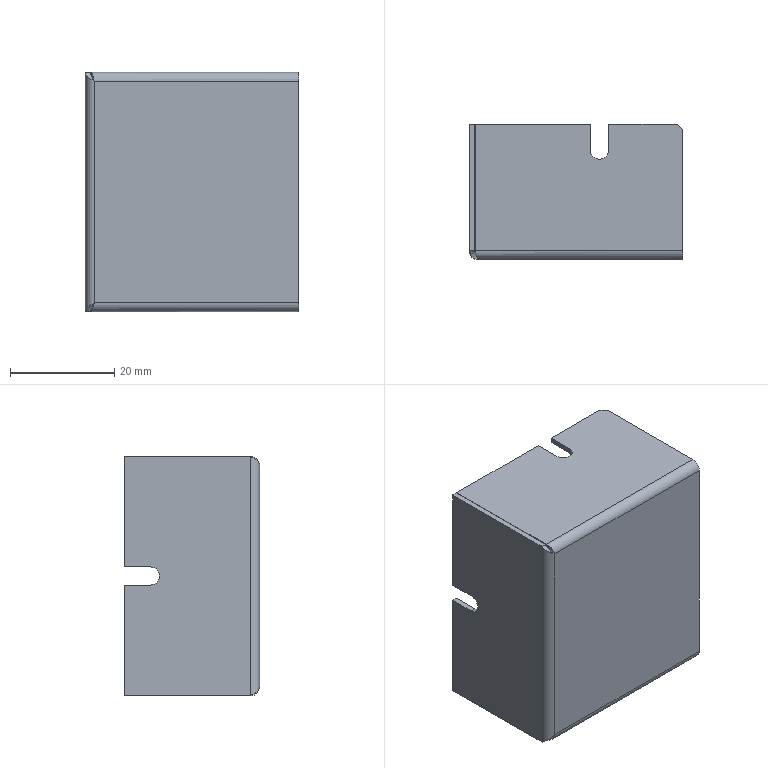Part | SolidWorks | features Chamfer 1, CornerFeat 1, Cut 1, EdgeFlange 1, FlatPattern 1, ICE 1, SMBaseFlange 1, SheetMetal 1 | 1 solid | 45 faces | box 41 x 26 x 46 mm | volume 4894 mm3 | plane 31 | cylinder 10 | spline 4 | commonest cylinder face diameters 3.5 x4 1.473 x3 3.473 x3
STEP:
#1=CARTESIAN_POINT('',(-20.,21.,23.75));
#2=VERTEX_POINT('',#1);
#3=CARTESIAN_POINT('',(-20.,19.25,22.));
#4=VERTEX_POINT('',#3);
#5=CARTESIAN_POINT('',(-20.,21.,22.));
#6=DIRECTION('',(1.,0.,0.));
#7=DIRECTION('',(0.,1.,0.));
#8=AXIS2_PLACEMENT_3D('',#5,#6,#7);
#9=CIRCLE('',#8,1.75);
#10=EDGE_CURVE('',#2,#4,#9,.T.);
#11=ORIENTED_EDGE('',*,*,#10,.T.);
#12=CARTESIAN_POINT('',(-21.,19.25,22.));
#13=VERTEX_POINT('',#12);
#14=CARTESIAN_POINT('',(-11.,19.25,22.));
#15=DIRECTION('',(-1.,0.,0.));
#16=VECTOR('',#15,1000.);
#17=LINE('',#14,#16);
#18=EDGE_CURVE('',#4,#13,#17,.T.);
#19=ORIENTED_EDGE('',*,*,#18,.T.);
#20=CARTESIAN_POINT('',(-21.,21.,23.75));
#21=VERTEX_POINT('',#20);
#22=CARTESIAN_POINT('',(-21.,21.,22.));
#23=DIRECTION('',(-1.,0.,0.));
#24=DIRECTION('',(0.,-1.,0.));
#25=AXIS2_PLACEMENT_3D('',#22,#23,#24);
#26=CIRCLE('',#25,1.75);
#27=EDGE_CURVE('',#13,#21,#26,.T.);
#28=ORIENTED_EDGE('',*,*,#27,.T.);
#29=CARTESIAN_POINT('',(-11.,21.,23.75));
#30=DIRECTION('',(-1.,0.,0.));
#31=VECTOR('',#30,1000.);
#32=LINE('',#29,#31);
#33=EDGE_CURVE('',#2,#21,#32,.T.);
#34=ORIENTED_EDGE('',*,*,#33,.F.);
#35=EDGE_LOOP('',(#11,#19,#28,#34));
#36=FACE_OUTER_BOUND('',#35,.T.);
#37=CARTESIAN_POINT('',(-11.,21.,22.));
#38=DIRECTION('',(-1.,0.,0.));
#39=DIRECTION('',(0.,-1.,0.));
#40=AXIS2_PLACEMENT_3D('',#37,#38,#39);
#41=CYLINDRICAL_SURFACE('',#40,1.75);
#42=ADVANCED_FACE('',(#36),#41,.F.);
#43=CARTESIAN_POINT('',(-20.,26.,45.));
#44=VERTEX_POINT('',#43);
#45=CARTESIAN_POINT('',(-20.,26.,23.75));
#46=VERTEX_POINT('',#45);
#47=CARTESIAN_POINT('',(-20.,26.,0.));
#48=DIRECTION('',(0.,0.,-1.));
#49=VECTOR('',#48,1000.);
#50=LINE('',#47,#49);
#51=EDGE_CURVE('',#44,#46,#50,.T.);
#52=ORIENTED_EDGE('',*,*,#51,.T.);
#53=CARTESIAN_POINT('',(-21.,26.,23.75));
#54=VERTEX_POINT('',#53);
#55=CARTESIAN_POINT('',(-21.,26.,23.75));
#56=DIRECTION('',(-1.,0.,0.));
#57=VECTOR('',#56,1000.);
#58=LINE('',#55,#57);
#59=EDGE_CURVE('',#46,#54,#58,.T.);
#60=ORIENTED_EDGE('',*,*,#59,.T.);
#61=CARTESIAN_POINT('',(-21.,26.,45.));
#62=VERTEX_POINT('',#61);
#63=CARTESIAN_POINT('',(-21.,26.,0.));
#64=DIRECTION('',(0.,0.,-1.));
#65=VECTOR('',#64,1000.);
#66=LINE('',#63,#65);
#67=EDGE_CURVE('',#62,#54,#66,.T.);
#68=ORIENTED_EDGE('',*,*,#67,.F.);
#69=CARTESIAN_POINT('',(-21.,26.,45.));
#70=DIRECTION('',(1.,0.,0.));
#71=VECTOR('',#70,1000.);
#72=LINE('',#69,#71);
#73=EDGE_CURVE('',#62,#44,#72,.T.);
#74=ORIENTED_EDGE('',*,*,#73,.T.);
#75=EDGE_LOOP('',(#52,#60,#68,#74));
#76=FACE_OUTER_BOUND('',#75,.T.);
#77=CARTESIAN_POINT('',(-21.,26.,0.));
#78=DIRECTION('',(0.,-1.,0.));
#79=DIRECTION('',(1.,0.,0.));
#80=AXIS2_PLACEMENT_3D('',#77,#78,#79);
#81=PLANE('',#80);
#82=ADVANCED_FACE('',(#76),#81,.F.);
#83=CARTESIAN_POINT('',(-19.9,26.,0.));
#84=VERTEX_POINT('',#83);
#85=CARTESIAN_POINT('',(2.25,26.,0.));
#86=VERTEX_POINT('',#85);
#87=CARTESIAN_POINT('',(20.,26.,0.));
#88=DIRECTION('',(1.,0.,0.));
#89=VECTOR('',#88,1000.);
#90=LINE('',#87,#89);
#91=EDGE_CURVE('',#84,#86,#90,.T.);
#92=ORIENTED_EDGE('',*,*,#91,.T.);
#93=CARTESIAN_POINT('',(2.25,26.,-1.));
#94=VERTEX_POINT('',#93);
#95=CARTESIAN_POINT('',(2.25,26.,-1.));
#96=DIRECTION('',(0.,0.,-1.));
#97=VECTOR('',#96,1000.);
#98=LINE('',#95,#97);
#99=EDGE_CURVE('',#86,#94,#98,.T.);
#100=ORIENTED_EDGE('',*,*,#99,.T.);
#101=CARTESIAN_POINT('',(-19.9,26.,-1.));
#102=VERTEX_POINT('',#101);
#103=CARTESIAN_POINT('',(20.,26.,-1.));
#104=DIRECTION('',(1.,0.,0.));
#105=VECTOR('',#104,1000.);
#106=LINE('',#103,#105);
#107=EDGE_CURVE('',#102,#94,#106,.T.);
#108=ORIENTED_EDGE('',*,*,#107,.F.);
#109=CARTESIAN_POINT('',(-19.9,26.,0.));
#110=DIRECTION('',(0.,0.,-1.));
#111=VECTOR('',#110,1000.);
#112=LINE('',#109,#111);
#113=EDGE_CURVE('',#84,#102,#112,.T.);
#114=ORIENTED_EDGE('',*,*,#113,.F.);
#115=EDGE_LOOP('',(#92,#100,#108,#114));
#116=FACE_OUTER_BOUND('',#115,.T.);
#117=CARTESIAN_POINT('',(20.,26.,-1.));
#118=DIRECTION('',(0.,-1.,0.));
#119=DIRECTION('',(0.,0.,-1.));
#120=AXIS2_PLACEMENT_3D('',#117,#118,#119);
#121=PLANE('',#120);
#122=ADVANCED_FACE('',(#116),#121,.F.);
#123=CARTESIAN_POINT('',(2.25,26.,45.));
#124=VERTEX_POINT('',#123);
#125=CARTESIAN_POINT('',(-19.9,26.,45.));
#126=VERTEX_POINT('',#125);
#127=CARTESIAN_POINT('',(-20.,26.,45.));
#128=DIRECTION('',(-1.,0.,0.));
#129=VECTOR('',#128,1000.);
#130=LINE('',#127,#129);
#131=EDGE_CURVE('',#124,#126,#130,.T.);
#132=ORIENTED_EDGE('',*,*,#131,.F.);
#133=CARTESIAN_POINT('',(2.25,26.,44.));
#134=VERTEX_POINT('',#133);
#135=CARTESIAN_POINT('',(2.25,26.,45.));
#136=DIRECTION('',(0.,0.,-1.));
#137=VECTOR('',#136,1000.);
#138=LINE('',#135,#137);
#139=EDGE_CURVE('',#124,#134,#138,.T.);
#140=ORIENTED_EDGE('',*,*,#139,.T.);
#141=CARTESIAN_POINT('',(-19.9,26.,44.));
#142=VERTEX_POINT('',#141);
#143=CARTESIAN_POINT('',(-20.,26.,44.));
#144=DIRECTION('',(-1.,0.,0.));
#145=VECTOR('',#144,1000.);
#146=LINE('',#143,#145);
#147=EDGE_CURVE('',#134,#142,#146,.T.);
#148=ORIENTED_EDGE('',*,*,#147,.T.);
#149=CARTESIAN_POINT('',(-19.9,26.,44.));
#150=DIRECTION('',(0.,0.,1.));
#151=VECTOR('',#150,1000.);
#152=LINE('',#149,#151);
#153=EDGE_CURVE('',#142,#126,#152,.T.);
#154=ORIENTED_EDGE('',*,*,#153,.T.);
#155=EDGE_LOOP('',(#132,#140,#148,#154));
#156=FACE_OUTER_BOUND('',#155,.T.);
#157=CARTESIAN_POINT('',(-20.,26.,45.));
#158=DIRECTION('',(0.,-1.,0.));
#159=DIRECTION('',(0.,0.,-1.));
#160=AXIS2_PLACEMENT_3D('',#157,#158,#159);
#161=PLANE('',#160);
#162=ADVANCED_FACE('',(#156),#161,.F.);
#163=CARTESIAN_POINT('',(-19.263,1.,43.263));
#164=VERTEX_POINT('',#163);
#165=CARTESIAN_POINT('',(-19.263,1.,0.7366));
#166=VERTEX_POINT('',#165);
#167=CARTESIAN_POINT('',(-19.263,1.,43.293));
#168=DIRECTION('',(0.,0.,-1.));
#169=VECTOR('',#168,1000.);
#170=LINE('',#167,#169);
#171=EDGE_CURVE('',#164,#166,#170,.T.);
#172=ORIENTED_EDGE('',*,*,#171,.F.);
#173=CARTESIAN_POINT('',(20.,1.,43.263));
#174=VERTEX_POINT('',#173);
#175=CARTESIAN_POINT('',(20.,1.,43.263));
#176=DIRECTION('',(-1.,0.,0.));
#177=VECTOR('',#176,1000.);
#178=LINE('',#175,#177);
#179=EDGE_CURVE('',#174,#164,#178,.T.);
#180=ORIENTED_EDGE('',*,*,#179,.F.);
#181=CARTESIAN_POINT('',(20.,1.,0.7366));
#182=VERTEX_POINT('',#181);
#183=CARTESIAN_POINT('',(20.,1.,44.));
#184=DIRECTION('',(0.,0.,-1.));
#185=VECTOR('',#184,1000.);
#186=LINE('',#183,#185);
#187=EDGE_CURVE('',#174,#182,#186,.T.);
#188=ORIENTED_EDGE('',*,*,#187,.T.);
#189=CARTESIAN_POINT('',(-19.293,1.,0.7366));
#190=DIRECTION('',(1.,0.,0.));
#191=VECTOR('',#190,1000.);
#192=LINE('',#189,#191);
#193=EDGE_CURVE('',#166,#182,#192,.T.);
#194=ORIENTED_EDGE('',*,*,#193,.F.);
#195=EDGE_LOOP('',(#172,#180,#188,#194));
#196=FACE_OUTER_BOUND('',#195,.T.);
#197=CARTESIAN_POINT('',(20.,1.,44.));
#198=DIRECTION('',(0.,-1.,0.));
#199=DIRECTION('',(0.,0.,-1.));
#200=AXIS2_PLACEMENT_3D('',#197,#198,#199);
#201=PLANE('',#200);
#202=ADVANCED_FACE('',(#196),#201,.F.);
#203=CARTESIAN_POINT('',(20.,0.,43.263));
#204=VERTEX_POINT('',#203);
#205=CARTESIAN_POINT('',(-19.263,0.,43.263));
#206=VERTEX_POINT('',#205);
#207=CARTESIAN_POINT('',(20.,0.,43.263));
#208=DIRECTION('',(-1.,0.,0.));
#209=VECTOR('',#208,1000.);
#210=LINE('',#207,#209);
#211=EDGE_CURVE('',#204,#206,#210,.T.);
#212=ORIENTED_EDGE('',*,*,#211,.T.);
#213=CARTESIAN_POINT('',(-19.263,0.,0.7366));
#214=VERTEX_POINT('',#213);
#215=CARTESIAN_POINT('',(-19.263,0.,43.293));
#216=DIRECTION('',(0.,0.,-1.));
#217=VECTOR('',#216,1000.);
#218=LINE('',#215,#217);
#219=EDGE_CURVE('',#206,#214,#218,.T.);
#220=ORIENTED_EDGE('',*,*,#219,.T.);
#221=CARTESIAN_POINT('',(20.,0.,0.7366));
#222=VERTEX_POINT('',#221);
#223=CARTESIAN_POINT('',(-19.293,0.,0.7366));
#224=DIRECTION('',(1.,0.,0.));
#225=VECTOR('',#224,1000.);
#226=LINE('',#223,#225);
#227=EDGE_CURVE('',#214,#222,#226,.T.);
#228=ORIENTED_EDGE('',*,*,#227,.T.);
#229=CARTESIAN_POINT('',(20.,0.,44.));
#230=DIRECTION('',(0.,0.,-1.));
#231=VECTOR('',#230,1000.);
#232=LINE('',#229,#231);
#233=EDGE_CURVE('',#204,#222,#232,.T.);
#234=ORIENTED_EDGE('',*,*,#233,.F.);
#235=EDGE_LOOP('',(#212,#220,#228,#234));
#236=FACE_OUTER_BOUND('',#235,.T.);
#237=CARTESIAN_POINT('',(20.,0.,44.));
#238=DIRECTION('',(0.,-1.,0.));
#239=DIRECTION('',(0.,0.,-1.));
#240=AXIS2_PLACEMENT_3D('',#237,#238,#239);
#241=PLANE('',#240);
#242=ADVANCED_FACE('',(#236),#241,.T.);
#243=ORIENTED_EDGE('',*,*,#187,.F.);
#244=CARTESIAN_POINT('',(20.,1.,43.263));
#245=DIRECTION('',(0.,-1.,0.));
#246=VECTOR('',#245,1000.);
#247=LINE('',#244,#246);
#248=EDGE_CURVE('',#174,#204,#247,.T.);
#249=ORIENTED_EDGE('',*,*,#248,.T.);
#250=ORIENTED_EDGE('',*,*,#233,.T.);
#251=CARTESIAN_POINT('',(20.,1.,0.7366));
#252=DIRECTION('',(0.,-1.,0.));
#253=VECTOR('',#252,1000.);
#254=LINE('',#251,#253);
#255=EDGE_CURVE('',#182,#222,#254,.T.);
#256=ORIENTED_EDGE('',*,*,#255,.F.);
#257=EDGE_LOOP('',(#243,#249,#250,#256));
#258=FACE_OUTER_BOUND('',#257,.T.);
#259=CARTESIAN_POINT('',(20.,1.,44.));
#260=DIRECTION('',(1.,0.,0.));
#261=DIRECTION('',(0.,0.,-1.));
#262=AXIS2_PLACEMENT_3D('',#259,#260,#261);
#263=PLANE('',#262);
#264=ADVANCED_FACE('',(#258),#263,.T.);
#265=CARTESIAN_POINT('',(20.,1.737,0.));
#266=VERTEX_POINT('',#265);
#267=CARTESIAN_POINT('',(20.,1.737,-1.));
#268=VERTEX_POINT('',#267);
#269=CARTESIAN_POINT('',(20.,1.737,0.));
#270=DIRECTION('',(0.,0.,-1.));
#271=VECTOR('',#270,1000.);
#272=LINE('',#269,#271);
#273=EDGE_CURVE('',#266,#268,#272,.T.);
#274=ORIENTED_EDGE('',*,*,#273,.F.);
#275=CARTESIAN_POINT('',(20.,1.737,0.7366));
#276=DIRECTION('',(-1.,0.,0.));
#277=DIRECTION('',(0.,0.,-1.));
#278=AXIS2_PLACEMENT_3D('',#275,#276,#277);
#279=CIRCLE('',#278,0.7366);
#280=EDGE_CURVE('',#266,#182,#279,.T.);
#281=ORIENTED_EDGE('',*,*,#280,.T.);
#282=ORIENTED_EDGE('',*,*,#255,.T.);
#283=CARTESIAN_POINT('',(20.,1.737,0.7366));
#284=DIRECTION('',(-1.,0.,0.));
#285=DIRECTION('',(0.,0.,1.));
#286=AXIS2_PLACEMENT_3D('',#283,#284,#285);
#287=CIRCLE('',#286,1.737);
#288=EDGE_CURVE('',#268,#222,#287,.T.);
#289=ORIENTED_EDGE('',*,*,#288,.F.);
#290=EDGE_LOOP('',(#274,#281,#282,#289));
#291=FACE_OUTER_BOUND('',#290,.T.);
#292=CARTESIAN_POINT('',(20.,1.737,0.7366));
#293=DIRECTION('',(1.,0.,0.));
#294=DIRECTION('',(0.,0.,-1.));
#295=AXIS2_PLACEMENT_3D('',#292,#293,#294);
#296=PLANE('',#295);
#297=ADVANCED_FACE('',(#291),#296,.T.);
#298=CARTESIAN_POINT('',(-19.9,1.737,0.));
#299=VERTEX_POINT('',#298);
#300=CARTESIAN_POINT('',(-19.263,1.,0.7366));
#301=CARTESIAN_POINT('',(-19.369,1.,0.5438));
#302=CARTESIAN_POINT('',(-19.476,1.079,0.3521));
#303=CARTESIAN_POINT('',(-19.688,1.352,0.07939));
#304=CARTESIAN_POINT('',(-19.794,1.544,0.));
#305=CARTESIAN_POINT('',(-19.9,1.737,0.));
#306=B_SPLINE_CURVE_WITH_KNOTS('',3,(#300,#301,#302,#303,#304,#305),.UNSPECIFIED.,.F.,.F.,(4,2,4),(0.,0.5,1.),.UNSPECIFIED.);
#307=EDGE_CURVE('',#166,#299,#306,.T.);
#308=ORIENTED_EDGE('',*,*,#307,.T.);
#309=CARTESIAN_POINT('',(-19.9,1.737,-1.));
#310=VERTEX_POINT('',#309);
#311=CARTESIAN_POINT('',(-19.9,1.737,0.));
#312=CARTESIAN_POINT('',(-19.9,1.737,-1.));
#313=B_SPLINE_CURVE_WITH_KNOTS('',1,(#311,#312),.UNSPECIFIED.,.F.,.F.,(2,2),(0.,1.),.UNSPECIFIED.);
#314=EDGE_CURVE('',#299,#310,#313,.T.);
#315=ORIENTED_EDGE('',*,*,#314,.T.);
#316=CARTESIAN_POINT('',(-19.263,0.,0.7366));
#317=CARTESIAN_POINT('',(-19.29,0.,0.622));
#318=CARTESIAN_POINT('',(-19.317,0.01124,0.5089));
#319=CARTESIAN_POINT('',(-19.37,0.05561,0.2861));
#320=CARTESIAN_POINT('',(-19.396,0.0892,0.1756));
#321=CARTESIAN_POINT('',(-19.449,0.176,-0.03353));
#322=CARTESIAN_POINT('',(-19.475,0.2293,-0.1332));
#323=CARTESIAN_POINT('',(-19.529,0.3557,-0.3226));
#324=CARTESIAN_POINT('',(-19.555,0.4287,-0.4114));
#325=CARTESIAN_POINT('',(-19.634,0.6684,-0.6511));
#326=CARTESIAN_POINT('',(-19.688,0.862,-0.7806));
#327=CARTESIAN_POINT('',(-19.793,1.28,-0.9539));
#328=CARTESIAN_POINT('',(-19.847,1.507,-1.));
#329=CARTESIAN_POINT('',(-19.9,1.737,-1.));
#330=B_SPLINE_CURVE_WITH_KNOTS('',3,(#316,#317,#318,#319,#320,#321,#322,#323,#324,#325,#326,#327,#328,#329),.UNSPECIFIED.,.F.,.F.,(4,2,2,2,2,2,4),(0.,0.0003495,0.0006991,0.001049,0.001398,0.002097,0.002796),.UNSPECIFIED.);
#331=EDGE_CURVE('',#214,#310,#330,.T.);
#332=ORIENTED_EDGE('',*,*,#331,.F.);
#333=CARTESIAN_POINT('',(-19.263,1.,0.7366));
#334=CARTESIAN_POINT('',(-19.263,0.,0.7366));
#335=B_SPLINE_CURVE_WITH_KNOTS('',1,(#333,#334),.UNSPECIFIED.,.F.,.F.,(2,2),(0.,1.),.UNSPECIFIED.);
#336=EDGE_CURVE('',#166,#214,#335,.T.);
#337=ORIENTED_EDGE('',*,*,#336,.F.);
#338=EDGE_LOOP('',(#308,#315,#332,#337));
#339=FACE_OUTER_BOUND('',#338,.T.);
#340=CARTESIAN_POINT('',(-19.263,-0.0101,0.7366));
#341=CARTESIAN_POINT('',(-19.316,-0.0101,0.5079));
#342=CARTESIAN_POINT('',(-19.37,0.03536,0.2794));
#343=CARTESIAN_POINT('',(-19.476,0.2104,-0.1431));
#344=CARTESIAN_POINT('',(-19.529,0.3398,-0.3368));
#345=CARTESIAN_POINT('',(-19.635,0.6632,-0.6602));
#346=CARTESIAN_POINT('',(-19.688,0.8569,-0.7896));
#347=CARTESIAN_POINT('',(-19.794,1.279,-0.9646));
#348=CARTESIAN_POINT('',(-19.847,1.508,-1.01));
#349=CARTESIAN_POINT('',(-19.9,1.737,-1.01));
#350=CARTESIAN_POINT('',(-19.263,0.,0.7366));
#351=CARTESIAN_POINT('',(-19.316,0.,0.5092));
#352=CARTESIAN_POINT('',(-19.37,0.0452,0.282));
#353=CARTESIAN_POINT('',(-19.476,0.2192,-0.138));
#354=CARTESIAN_POINT('',(-19.529,0.3479,-0.3306));
#355=CARTESIAN_POINT('',(-19.635,0.6694,-0.6521));
#356=CARTESIAN_POINT('',(-19.688,0.862,-0.7808));
#357=CARTESIAN_POINT('',(-19.794,1.282,-0.9548));
#358=CARTESIAN_POINT('',(-19.847,1.509,-1.));
#359=CARTESIAN_POINT('',(-19.9,1.737,-1.));
#360=CARTESIAN_POINT('',(-19.263,1.,0.7366));
#361=CARTESIAN_POINT('',(-19.316,1.,0.6402));
#362=CARTESIAN_POINT('',(-19.37,1.019,0.5438));
#363=CARTESIAN_POINT('',(-19.476,1.093,0.3656));
#364=CARTESIAN_POINT('',(-19.529,1.148,0.2839));
#365=CARTESIAN_POINT('',(-19.635,1.284,0.1476));
#366=CARTESIAN_POINT('',(-19.688,1.366,0.09297));
#367=CARTESIAN_POINT('',(-19.794,1.544,0.01917));
#368=CARTESIAN_POINT('',(-19.847,1.64,0.));
#369=CARTESIAN_POINT('',(-19.9,1.737,0.));
#370=CARTESIAN_POINT('',(-19.263,1.01,0.7366));
#371=CARTESIAN_POINT('',(-19.316,1.01,0.6415));
#372=CARTESIAN_POINT('',(-19.37,1.029,0.5464));
#373=CARTESIAN_POINT('',(-19.476,1.102,0.3707));
#374=CARTESIAN_POINT('',(-19.529,1.156,0.2901));
#375=CARTESIAN_POINT('',(-19.635,1.29,0.1556));
#376=CARTESIAN_POINT('',(-19.688,1.371,0.1017));
#377=CARTESIAN_POINT('',(-19.794,1.546,0.02891));
#378=CARTESIAN_POINT('',(-19.847,1.641,0.01));
#379=CARTESIAN_POINT('',(-19.9,1.737,0.01));
#380=B_SPLINE_SURFACE_WITH_KNOTS('',1,3,((#340,#341,#342,#343,#344,#345,#346,#347,#348,#349),(#350,#351,#352,#353,#354,#355,#356,#357,#358,#359),(#360,#361,#362,#363,#364,#365,#366,#367,#368,#369),(#370,#371,#372,#373,#374,#375,#376,#377,#378,#379)),.UNSPECIFIED.,.F.,.F.,.F.,(2,1,1,2),(4,2,2,2,4),(-0.0101,0.,1.,1.01),(0.,0.25,0.5,0.75,1.),.UNSPECIFIED.);
#381=ADVANCED_FACE('',(#339),#380,.T.);
#382=ORIENTED_EDGE('',*,*,#227,.F.);
#383=ORIENTED_EDGE('',*,*,#331,.T.);
#384=CARTESIAN_POINT('',(0.,1.737,-1.));
#385=DIRECTION('',(1.,0.,0.));
#386=VECTOR('',#385,1000.);
#387=LINE('',#384,#386);
#388=EDGE_CURVE('',#310,#268,#387,.T.);
#389=ORIENTED_EDGE('',*,*,#388,.T.);
#390=ORIENTED_EDGE('',*,*,#288,.T.);
#391=EDGE_LOOP('',(#382,#383,#389,#390));
#392=FACE_OUTER_BOUND('',#391,.T.);
#393=CARTESIAN_POINT('',(-39.591,1.737,0.7366));
#394=DIRECTION('',(1.,0.,0.));
#395=DIRECTION('',(0.,0.,-1.));
#396=AXIS2_PLACEMENT_3D('',#393,#394,#395);
#397=CYLINDRICAL_SURFACE('',#396,1.737);
#398=ADVANCED_FACE('',(#392),#397,.T.);
#399=ORIENTED_EDGE('',*,*,#193,.T.);
#400=ORIENTED_EDGE('',*,*,#280,.F.);
#401=CARTESIAN_POINT('',(20.,1.737,0.));
#402=DIRECTION('',(-1.,0.,0.));
#403=VECTOR('',#402,1000.);
#404=LINE('',#401,#403);
#405=EDGE_CURVE('',#266,#299,#404,.T.);
#406=ORIENTED_EDGE('',*,*,#405,.T.);
#407=ORIENTED_EDGE('',*,*,#307,.F.);
#408=EDGE_LOOP('',(#399,#400,#406,#407));
#409=FACE_OUTER_BOUND('',#408,.T.);
#410=CARTESIAN_POINT('',(-39.591,1.737,0.7366));
#411=DIRECTION('',(1.,0.,0.));
#412=DIRECTION('',(0.,0.,-1.));
#413=AXIS2_PLACEMENT_3D('',#410,#411,#412);
#414=CYLINDRICAL_SURFACE('',#413,0.7366);
#415=ADVANCED_FACE('',(#409),#414,.F.);
#416=CARTESIAN_POINT('',(5.75,26.,0.));
#417=VERTEX_POINT('',#416);
#418=CARTESIAN_POINT('',(19.,26.,0.));
#419=VERTEX_POINT('',#418);
#420=CARTESIAN_POINT('',(20.,26.,0.));
#421=DIRECTION('',(1.,0.,0.));
#422=VECTOR('',#421,1000.);
#423=LINE('',#420,#422);
#424=EDGE_CURVE('',#417,#419,#423,.T.);
#425=ORIENTED_EDGE('',*,*,#424,.T.);
#426=CARTESIAN_POINT('',(19.,26.,-1.));
#427=VERTEX_POINT('',#426);
#428=CARTESIAN_POINT('',(19.,26.,-1.));
#429=DIRECTION('',(0.,0.,-1.));
#430=VECTOR('',#429,1000.);
#431=LINE('',#428,#430);
#432=EDGE_CURVE('',#419,#427,#431,.T.);
#433=ORIENTED_EDGE('',*,*,#432,.T.);
#434=CARTESIAN_POINT('',(5.75,26.,-1.));
#435=VERTEX_POINT('',#434);
#436=CARTESIAN_POINT('',(20.,26.,-1.));
#437=DIRECTION('',(1.,0.,0.));
#438=VECTOR('',#437,1000.);
#439=LINE('',#436,#438);
#440=EDGE_CURVE('',#435,#427,#439,.T.);
#441=ORIENTED_EDGE('',*,*,#440,.F.);
#442=CARTESIAN_POINT('',(5.75,26.,-1.));
#443=DIRECTION('',(0.,0.,1.));
#444=VECTOR('',#443,1000.);
#445=LINE('',#442,#444);
#446=EDGE_CURVE('',#435,#417,#445,.T.);
#447=ORIENTED_EDGE('',*,*,#446,.T.);
#448=EDGE_LOOP('',(#425,#433,#441,#447));
#449=FACE_OUTER_BOUND('',#448,.T.);
#450=CARTESIAN_POINT('',(20.,26.,-1.));
#451=DIRECTION('',(0.,-1.,0.));
#452=DIRECTION('',(0.,0.,-1.));
#453=AXIS2_PLACEMENT_3D('',#450,#451,#452);
#454=PLANE('',#453);
#455=ADVANCED_FACE('',(#449),#454,.F.);
#456=ORIENTED_EDGE('',*,*,#440,.T.);
#457=CARTESIAN_POINT('',(20.,25.,-1.));
#458=VERTEX_POINT('',#457);
#459=CARTESIAN_POINT('',(20.,25.,-1.));
#460=DIRECTION('',(0.7071,-0.7071,0.));
#461=VECTOR('',#460,1000.);
#462=LINE('',#459,#461);
#463=EDGE_CURVE('',#427,#458,#462,.T.);
#464=ORIENTED_EDGE('',*,*,#463,.T.);
#465=CARTESIAN_POINT('',(20.,1.,-1.));
#466=DIRECTION('',(0.,-1.,0.));
#467=VECTOR('',#466,1000.);
#468=LINE('',#465,#467);
#469=EDGE_CURVE('',#458,#268,#468,.T.);
#470=ORIENTED_EDGE('',*,*,#469,.T.);
#471=ORIENTED_EDGE('',*,*,#388,.F.);
#472=CARTESIAN_POINT('',(-19.9,1.737,-1.));
#473=DIRECTION('',(0.,1.,0.));
#474=VECTOR('',#473,1000.);
#475=LINE('',#472,#474);
#476=EDGE_CURVE('',#310,#102,#475,.T.);
#477=ORIENTED_EDGE('',*,*,#476,.T.);
#478=ORIENTED_EDGE('',*,*,#107,.T.);
#479=CARTESIAN_POINT('',(2.25,21.,-1.));
#480=VERTEX_POINT('',#479);
#481=CARTESIAN_POINT('',(2.25,0.,-1.));
#482=DIRECTION('',(0.,-1.,0.));
#483=VECTOR('',#482,1000.);
#484=LINE('',#481,#483);
#485=EDGE_CURVE('',#94,#480,#484,.T.);
#486=ORIENTED_EDGE('',*,*,#485,.T.);
#487=CARTESIAN_POINT('',(5.75,21.,-1.));
#488=VERTEX_POINT('',#487);
#489=CARTESIAN_POINT('',(4.,21.,-1.));
#490=DIRECTION('',(0.,0.,1.));
#491=DIRECTION('',(0.,-1.,0.));
#492=AXIS2_PLACEMENT_3D('',#489,#490,#491);
#493=CIRCLE('',#492,1.75);
#494=EDGE_CURVE('',#480,#488,#493,.T.);
#495=ORIENTED_EDGE('',*,*,#494,.T.);
#496=CARTESIAN_POINT('',(5.75,0.,-1.));
#497=DIRECTION('',(0.,1.,0.));
#498=VECTOR('',#497,1000.);
#499=LINE('',#496,#498);
#500=EDGE_CURVE('',#488,#435,#499,.T.);
#501=ORIENTED_EDGE('',*,*,#500,.T.);
#502=EDGE_LOOP('',(#456,#464,#470,#471,#477,#478,#486,#495,#501));
#503=FACE_OUTER_BOUND('',#502,.T.);
#504=CARTESIAN_POINT('',(0.,0.,-1.));
#505=DIRECTION('',(0.,0.,1.));
#506=DIRECTION('',(0.,-1.,0.));
#507=AXIS2_PLACEMENT_3D('',#504,#505,#506);
#508=PLANE('',#507);
#509=ADVANCED_FACE('',(#503),#508,.F.);
#510=ORIENTED_EDGE('',*,*,#476,.F.);
#511=ORIENTED_EDGE('',*,*,#314,.F.);
#512=CARTESIAN_POINT('',(-19.9,1.737,0.));
#513=DIRECTION('',(0.,1.,0.));
#514=VECTOR('',#513,1000.);
#515=LINE('',#512,#514);
#516=EDGE_CURVE('',#299,#84,#515,.T.);
#517=ORIENTED_EDGE('',*,*,#516,.T.);
#518=ORIENTED_EDGE('',*,*,#113,.T.);
#519=EDGE_LOOP('',(#510,#511,#517,#518));
#520=FACE_OUTER_BOUND('',#519,.T.);
#521=CARTESIAN_POINT('',(-19.9,1.737,0.));
#522=DIRECTION('',(-1.,0.,0.));
#523=DIRECTION('',(0.,-1.,0.));
#524=AXIS2_PLACEMENT_3D('',#521,#522,#523);
#525=PLANE('',#524);
#526=ADVANCED_FACE('',(#520),#525,.T.);
#527=CARTESIAN_POINT('',(20.,25.,0.));
#528=VERTEX_POINT('',#527);
#529=CARTESIAN_POINT('',(20.,1.,0.));
#530=DIRECTION('',(0.,-1.,0.));
#531=VECTOR('',#530,1000.);
#532=LINE('',#529,#531);
#533=EDGE_CURVE('',#528,#266,#532,.T.);
#534=ORIENTED_EDGE('',*,*,#533,.F.);
#535=CARTESIAN_POINT('',(22.5,22.5,0.));
#536=DIRECTION('',(-0.7071,0.7071,0.));
#537=VECTOR('',#536,1000.);
#538=LINE('',#535,#537);
#539=EDGE_CURVE('',#528,#419,#538,.T.);
#540=ORIENTED_EDGE('',*,*,#539,.T.);
#541=ORIENTED_EDGE('',*,*,#424,.F.);
#542=CARTESIAN_POINT('',(5.75,21.,0.));
#543=VERTEX_POINT('',#542);
#544=CARTESIAN_POINT('',(5.75,0.,0.));
#545=DIRECTION('',(0.,1.,0.));
#546=VECTOR('',#545,1000.);
#547=LINE('',#544,#546);
#548=EDGE_CURVE('',#543,#417,#547,.T.);
#549=ORIENTED_EDGE('',*,*,#548,.F.);
#550=CARTESIAN_POINT('',(2.25,21.,0.));
#551=VERTEX_POINT('',#550);
#552=CARTESIAN_POINT('',(4.,21.,0.));
#553=DIRECTION('',(0.,0.,1.));
#554=DIRECTION('',(0.,-1.,0.));
#555=AXIS2_PLACEMENT_3D('',#552,#553,#554);
#556=CIRCLE('',#555,1.75);
#557=EDGE_CURVE('',#551,#543,#556,.T.);
#558=ORIENTED_EDGE('',*,*,#557,.F.);
#559=CARTESIAN_POINT('',(2.25,0.,0.));
#560=DIRECTION('',(0.,-1.,0.));
#561=VECTOR('',#560,1000.);
#562=LINE('',#559,#561);
#563=EDGE_CURVE('',#86,#551,#562,.T.);
#564=ORIENTED_EDGE('',*,*,#563,.F.);
#565=ORIENTED_EDGE('',*,*,#91,.F.);
#566=ORIENTED_EDGE('',*,*,#516,.F.);
#567=ORIENTED_EDGE('',*,*,#405,.F.);
#568=EDGE_LOOP('',(#534,#540,#541,#549,#558,#564,#565,#566,#567));
#569=FACE_OUTER_BOUND('',#568,.T.);
#570=CARTESIAN_POINT('',(0.,0.,0.));
#571=DIRECTION('',(0.,0.,1.));
#572=DIRECTION('',(0.,-1.,0.));
#573=AXIS2_PLACEMENT_3D('',#570,#571,#572);
#574=PLANE('',#573);
#575=ADVANCED_FACE('',(#569),#574,.T.);
#576=ORIENTED_EDGE('',*,*,#469,.F.);
#577=CARTESIAN_POINT('',(20.,25.,-1.));
#578=DIRECTION('',(0.,0.,1.));
#579=VECTOR('',#578,1000.);
#580=LINE('',#577,#579);
#581=EDGE_CURVE('',#458,#528,#580,.T.);
#582=ORIENTED_EDGE('',*,*,#581,.T.);
#583=ORIENTED_EDGE('',*,*,#533,.T.);
#584=ORIENTED_EDGE('',*,*,#273,.T.);
#585=EDGE_LOOP('',(#576,#582,#583,#584));
#586=FACE_OUTER_BOUND('',#585,.T.);
#587=CARTESIAN_POINT('',(20.,1.,-1.));
#588=DIRECTION('',(-1.,0.,0.));
#589=DIRECTION('',(0.,0.,1.));
#590=AXIS2_PLACEMENT_3D('',#587,#588,#589);
#591=PLANE('',#590);
#592=ADVANCED_FACE('',(#586),#591,.F.);
#593=CARTESIAN_POINT('',(-19.9,1.737,44.));
#594=VERTEX_POINT('',#593);
#595=CARTESIAN_POINT('',(-19.9,1.737,45.));
#596=VERTEX_POINT('',#595);
#597=CARTESIAN_POINT('',(-19.9,1.737,44.));
#598=CARTESIAN_POINT('',(-19.9,1.737,44.333));
#599=CARTESIAN_POINT('',(-19.9,1.737,44.667));
#600=CARTESIAN_POINT('',(-19.9,1.737,45.));
#601=B_SPLINE_CURVE_WITH_KNOTS('',3,(#597,#598,#599,#600),.UNSPECIFIED.,.F.,.F.,(4,4),(0.,1.),.UNSPECIFIED.);
#602=EDGE_CURVE('',#594,#596,#601,.T.);
#603=ORIENTED_EDGE('',*,*,#602,.F.);
#604=CARTESIAN_POINT('',(-19.9,1.737,44.));
#605=CARTESIAN_POINT('',(-19.794,1.544,44.));
#606=CARTESIAN_POINT('',(-19.688,1.352,43.921));
#607=CARTESIAN_POINT('',(-19.476,1.079,43.648));
#608=CARTESIAN_POINT('',(-19.37,1.,43.456));
#609=CARTESIAN_POINT('',(-19.263,1.,43.263));
#610=B_SPLINE_CURVE_WITH_KNOTS('',3,(#604,#605,#606,#607,#608,#609),.UNSPECIFIED.,.F.,.F.,(4,2,4),(0.,0.5,1.),.UNSPECIFIED.);
#611=EDGE_CURVE('',#594,#164,#610,.T.);
#612=ORIENTED_EDGE('',*,*,#611,.T.);
#613=CARTESIAN_POINT('',(-19.263,1.,43.263));
#614=CARTESIAN_POINT('',(-19.263,0.,43.263));
#615=B_SPLINE_CURVE_WITH_KNOTS('',1,(#613,#614),.UNSPECIFIED.,.F.,.F.,(2,2),(0.,1.),.UNSPECIFIED.);
#616=EDGE_CURVE('',#164,#206,#615,.T.);
#617=ORIENTED_EDGE('',*,*,#616,.T.);
#618=CARTESIAN_POINT('',(-19.9,1.737,45.));
#619=CARTESIAN_POINT('',(-19.873,1.622,45.));
#620=CARTESIAN_POINT('',(-19.847,1.509,44.989));
#621=CARTESIAN_POINT('',(-19.794,1.286,44.944));
#622=CARTESIAN_POINT('',(-19.767,1.176,44.911));
#623=CARTESIAN_POINT('',(-19.688,0.8619,44.781));
#624=CARTESIAN_POINT('',(-19.634,0.6685,44.651));
#625=CARTESIAN_POINT('',(-19.529,0.3489,44.332));
#626=CARTESIAN_POINT('',(-19.476,0.2194,44.138));
#627=CARTESIAN_POINT('',(-19.37,0.04605,43.72));
#628=CARTESIAN_POINT('',(-19.317,0.,43.493));
#629=CARTESIAN_POINT('',(-19.263,0.,43.263));
#630=B_SPLINE_CURVE_WITH_KNOTS('',3,(#618,#619,#620,#621,#622,#623,#624,#625,#626,#627,#628,#629),.UNSPECIFIED.,.F.,.F.,(4,2,2,2,2,4),(0.,0.0003496,0.0006992,0.001398,0.002098,0.002797),.UNSPECIFIED.);
#631=EDGE_CURVE('',#596,#206,#630,.T.);
#632=ORIENTED_EDGE('',*,*,#631,.F.);
#633=EDGE_LOOP('',(#603,#612,#617,#632));
#634=FACE_OUTER_BOUND('',#633,.T.);
#635=CARTESIAN_POINT('',(-19.9,1.737,45.01));
#636=CARTESIAN_POINT('',(-19.847,1.508,45.01));
#637=CARTESIAN_POINT('',(-19.794,1.279,44.965));
#638=CARTESIAN_POINT('',(-19.688,0.857,44.79));
#639=CARTESIAN_POINT('',(-19.635,0.6632,44.66));
#640=CARTESIAN_POINT('',(-19.529,0.3399,44.337));
#641=CARTESIAN_POINT('',(-19.476,0.2104,44.143));
#642=CARTESIAN_POINT('',(-19.37,0.03546,43.721));
#643=CARTESIAN_POINT('',(-19.316,-0.01,43.492));
#644=CARTESIAN_POINT('',(-19.263,-0.01,43.263));
#645=CARTESIAN_POINT('',(-19.9,1.737,45.));
#646=CARTESIAN_POINT('',(-19.847,1.509,45.));
#647=CARTESIAN_POINT('',(-19.794,1.282,44.955));
#648=CARTESIAN_POINT('',(-19.688,0.862,44.781));
#649=CARTESIAN_POINT('',(-19.635,0.6694,44.652));
#650=CARTESIAN_POINT('',(-19.529,0.3479,44.331));
#651=CARTESIAN_POINT('',(-19.476,0.2192,44.138));
#652=CARTESIAN_POINT('',(-19.37,0.0452,43.718));
#653=CARTESIAN_POINT('',(-19.316,0.,43.491));
#654=CARTESIAN_POINT('',(-19.263,0.,43.263));
#655=CARTESIAN_POINT('',(-19.9,1.737,44.));
#656=CARTESIAN_POINT('',(-19.847,1.64,44.));
#657=CARTESIAN_POINT('',(-19.794,1.544,43.981));
#658=CARTESIAN_POINT('',(-19.688,1.366,43.907));
#659=CARTESIAN_POINT('',(-19.635,1.284,43.852));
#660=CARTESIAN_POINT('',(-19.529,1.148,43.716));
#661=CARTESIAN_POINT('',(-19.476,1.093,43.634));
#662=CARTESIAN_POINT('',(-19.37,1.019,43.456));
#663=CARTESIAN_POINT('',(-19.316,1.,43.36));
#664=CARTESIAN_POINT('',(-19.263,1.,43.263));
#665=CARTESIAN_POINT('',(-19.9,1.737,43.99));
#666=CARTESIAN_POINT('',(-19.847,1.641,43.99));
#667=CARTESIAN_POINT('',(-19.794,1.546,43.971));
#668=CARTESIAN_POINT('',(-19.688,1.371,43.898));
#669=CARTESIAN_POINT('',(-19.635,1.29,43.844));
#670=CARTESIAN_POINT('',(-19.529,1.156,43.71));
#671=CARTESIAN_POINT('',(-19.476,1.102,43.629));
#672=CARTESIAN_POINT('',(-19.37,1.029,43.454));
#673=CARTESIAN_POINT('',(-19.316,1.01,43.359));
#674=CARTESIAN_POINT('',(-19.263,1.01,43.263));
#675=B_SPLINE_SURFACE_WITH_KNOTS('',1,3,((#635,#636,#637,#638,#639,#640,#641,#642,#643,#644),(#645,#646,#647,#648,#649,#650,#651,#652,#653,#654),(#655,#656,#657,#658,#659,#660,#661,#662,#663,#664),(#665,#666,#667,#668,#669,#670,#671,#672,#673,#674)),.UNSPECIFIED.,.F.,.F.,.F.,(2,1,1,2),(4,2,2,2,4),(-0.01,0.,1.,1.01),(0.,0.25,0.5,0.75,1.),.UNSPECIFIED.);
#676=ADVANCED_FACE('',(#634),#675,.T.);
#677=CARTESIAN_POINT('',(20.,1.737,44.));
#678=VERTEX_POINT('',#677);
#679=CARTESIAN_POINT('',(20.,1.737,43.263));
#680=DIRECTION('',(-1.,0.,0.));
#681=DIRECTION('',(0.,0.,1.));
#682=AXIS2_PLACEMENT_3D('',#679,#680,#681);
#683=CIRCLE('',#682,0.7366);
#684=EDGE_CURVE('',#174,#678,#683,.T.);
#685=ORIENTED_EDGE('',*,*,#684,.T.);
#686=CARTESIAN_POINT('',(20.,1.737,45.));
#687=VERTEX_POINT('',#686);
#688=CARTESIAN_POINT('',(20.,1.737,44.));
#689=DIRECTION('',(0.,0.,1.));
#690=VECTOR('',#689,1000.);
#691=LINE('',#688,#690);
#692=EDGE_CURVE('',#678,#687,#691,.T.);
#693=ORIENTED_EDGE('',*,*,#692,.T.);
#694=CARTESIAN_POINT('',(20.,1.737,43.263));
#695=DIRECTION('',(-1.,0.,0.));
#696=DIRECTION('',(0.,0.,1.));
#697=AXIS2_PLACEMENT_3D('',#694,#695,#696);
#698=CIRCLE('',#697,1.737);
#699=EDGE_CURVE('',#204,#687,#698,.T.);
#700=ORIENTED_EDGE('',*,*,#699,.F.);
#701=ORIENTED_EDGE('',*,*,#248,.F.);
#702=EDGE_LOOP('',(#685,#693,#700,#701));
#703=FACE_OUTER_BOUND('',#702,.T.);
#704=CARTESIAN_POINT('',(20.,1.737,43.263));
#705=DIRECTION('',(1.,0.,0.));
#706=DIRECTION('',(0.,0.,-1.));
#707=AXIS2_PLACEMENT_3D('',#704,#705,#706);
#708=PLANE('',#707);
#709=ADVANCED_FACE('',(#703),#708,.T.);
#710=ORIENTED_EDGE('',*,*,#211,.F.);
#711=ORIENTED_EDGE('',*,*,#699,.T.);
#712=CARTESIAN_POINT('',(0.,1.737,45.));
#713=DIRECTION('',(-1.,0.,0.));
#714=VECTOR('',#713,1000.);
#715=LINE('',#712,#714);
#716=EDGE_CURVE('',#687,#596,#715,.T.);
#717=ORIENTED_EDGE('',*,*,#716,.T.);
#718=ORIENTED_EDGE('',*,*,#631,.T.);
#719=EDGE_LOOP('',(#710,#711,#717,#718));
#720=FACE_OUTER_BOUND('',#719,.T.);
#721=CARTESIAN_POINT('',(40.328,1.737,43.263));
#722=DIRECTION('',(-1.,0.,0.));
#723=DIRECTION('',(0.,0.,1.));
#724=AXIS2_PLACEMENT_3D('',#721,#722,#723);
#725=CYLINDRICAL_SURFACE('',#724,1.737);
#726=ADVANCED_FACE('',(#720),#725,.T.);
#727=ORIENTED_EDGE('',*,*,#179,.T.);
#728=ORIENTED_EDGE('',*,*,#611,.F.);
#729=CARTESIAN_POINT('',(-20.,1.737,44.));
#730=DIRECTION('',(1.,0.,0.));
#731=VECTOR('',#730,1000.);
#732=LINE('',#729,#731);
#733=EDGE_CURVE('',#594,#678,#732,.T.);
#734=ORIENTED_EDGE('',*,*,#733,.T.);
#735=ORIENTED_EDGE('',*,*,#684,.F.);
#736=EDGE_LOOP('',(#727,#728,#734,#735));
#737=FACE_OUTER_BOUND('',#736,.T.);
#738=CARTESIAN_POINT('',(40.328,1.737,43.263));
#739=DIRECTION('',(-1.,0.,0.));
#740=DIRECTION('',(0.,0.,1.));
#741=AXIS2_PLACEMENT_3D('',#738,#739,#740);
#742=CYLINDRICAL_SURFACE('',#741,0.7366);
#743=ADVANCED_FACE('',(#737),#742,.F.);
#744=CARTESIAN_POINT('',(19.,26.,45.));
#745=VERTEX_POINT('',#744);
#746=CARTESIAN_POINT('',(5.75,26.,45.));
#747=VERTEX_POINT('',#746);
#748=CARTESIAN_POINT('',(-20.,26.,45.));
#749=DIRECTION('',(-1.,0.,0.));
#750=VECTOR('',#749,1000.);
#751=LINE('',#748,#750);
#752=EDGE_CURVE('',#745,#747,#751,.T.);
#753=ORIENTED_EDGE('',*,*,#752,.F.);
#754=CARTESIAN_POINT('',(19.,26.,44.));
#755=VERTEX_POINT('',#754);
#756=CARTESIAN_POINT('',(19.,26.,45.));
#757=DIRECTION('',(0.,0.,-1.));
#758=VECTOR('',#757,1000.);
#759=LINE('',#756,#758);
#760=EDGE_CURVE('',#745,#755,#759,.T.);
#761=ORIENTED_EDGE('',*,*,#760,.T.);
#762=CARTESIAN_POINT('',(5.75,26.,44.));
#763=VERTEX_POINT('',#762);
#764=CARTESIAN_POINT('',(-20.,26.,44.));
#765=DIRECTION('',(-1.,0.,0.));
#766=VECTOR('',#765,1000.);
#767=LINE('',#764,#766);
#768=EDGE_CURVE('',#755,#763,#767,.T.);
#769=ORIENTED_EDGE('',*,*,#768,.T.);
#770=CARTESIAN_POINT('',(5.75,26.,45.));
#771=DIRECTION('',(0.,0.,1.));
#772=VECTOR('',#771,1000.);
#773=LINE('',#770,#772);
#774=EDGE_CURVE('',#763,#747,#773,.T.);
#775=ORIENTED_EDGE('',*,*,#774,.T.);
#776=EDGE_LOOP('',(#753,#761,#769,#775));
#777=FACE_OUTER_BOUND('',#776,.T.);
#778=CARTESIAN_POINT('',(-20.,26.,45.));
#779=DIRECTION('',(0.,-1.,0.));
#780=DIRECTION('',(0.,0.,-1.));
#781=AXIS2_PLACEMENT_3D('',#778,#779,#780);
#782=PLANE('',#781);
#783=ADVANCED_FACE('',(#777),#782,.F.);
#784=CARTESIAN_POINT('',(20.,25.,45.));
#785=VERTEX_POINT('',#784);
#786=CARTESIAN_POINT('',(20.,26.,45.));
#787=DIRECTION('',(0.,1.,0.));
#788=VECTOR('',#787,1000.);
#789=LINE('',#786,#788);
#790=EDGE_CURVE('',#687,#785,#789,.T.);
#791=ORIENTED_EDGE('',*,*,#790,.T.);
#792=CARTESIAN_POINT('',(19.,26.,45.));
#793=DIRECTION('',(-0.7071,0.7071,0.));
#794=VECTOR('',#793,1000.);
#795=LINE('',#792,#794);
#796=EDGE_CURVE('',#785,#745,#795,.T.);
#797=ORIENTED_EDGE('',*,*,#796,.T.);
#798=ORIENTED_EDGE('',*,*,#752,.T.);
#799=CARTESIAN_POINT('',(5.75,21.,45.));
#800=VERTEX_POINT('',#799);
#801=CARTESIAN_POINT('',(5.75,21.,45.));
#802=DIRECTION('',(0.,1.,0.));
#803=VECTOR('',#802,1000.);
#804=LINE('',#801,#803);
#805=EDGE_CURVE('',#800,#747,#804,.T.);
#806=ORIENTED_EDGE('',*,*,#805,.F.);
#807=CARTESIAN_POINT('',(2.25,21.,45.));
#808=VERTEX_POINT('',#807);
#809=CARTESIAN_POINT('',(4.,21.,45.));
#810=DIRECTION('',(0.,0.,1.));
#811=DIRECTION('',(1.,0.,0.));
#812=AXIS2_PLACEMENT_3D('',#809,#810,#811);
#813=CIRCLE('',#812,1.75);
#814=EDGE_CURVE('',#808,#800,#813,.T.);
#815=ORIENTED_EDGE('',*,*,#814,.F.);
#816=CARTESIAN_POINT('',(2.25,21.,45.));
#817=DIRECTION('',(0.,-1.,0.));
#818=VECTOR('',#817,1000.);
#819=LINE('',#816,#818);
#820=EDGE_CURVE('',#124,#808,#819,.T.);
#821=ORIENTED_EDGE('',*,*,#820,.F.);
#822=ORIENTED_EDGE('',*,*,#131,.T.);
#823=CARTESIAN_POINT('',(-19.9,1.737,45.));
#824=DIRECTION('',(0.,1.,0.));
#825=VECTOR('',#824,1000.);
#826=LINE('',#823,#825);
#827=EDGE_CURVE('',#596,#126,#826,.T.);
#828=ORIENTED_EDGE('',*,*,#827,.F.);
#829=ORIENTED_EDGE('',*,*,#716,.F.);
#830=EDGE_LOOP('',(#791,#797,#798,#806,#815,#821,#822,#828,#829));
#831=FACE_OUTER_BOUND('',#830,.T.);
#832=CARTESIAN_POINT('',(0.,0.,45.));
#833=DIRECTION('',(0.,0.,-1.));
#834=DIRECTION('',(-1.,0.,0.));
#835=AXIS2_PLACEMENT_3D('',#832,#833,#834);
#836=PLANE('',#835);
#837=ADVANCED_FACE('',(#831),#836,.F.);
#838=CARTESIAN_POINT('',(20.,25.,44.));
#839=VERTEX_POINT('',#838);
#840=CARTESIAN_POINT('',(20.,26.,44.));
#841=DIRECTION('',(0.,1.,0.));
#842=VECTOR('',#841,1000.);
#843=LINE('',#840,#842);
#844=EDGE_CURVE('',#678,#839,#843,.T.);
#845=ORIENTED_EDGE('',*,*,#844,.T.);
#846=CARTESIAN_POINT('',(20.,25.,45.));
#847=DIRECTION('',(0.,0.,1.));
#848=VECTOR('',#847,1000.);
#849=LINE('',#846,#848);
#850=EDGE_CURVE('',#839,#785,#849,.T.);
#851=ORIENTED_EDGE('',*,*,#850,.T.);
#852=ORIENTED_EDGE('',*,*,#790,.F.);
#853=ORIENTED_EDGE('',*,*,#692,.F.);
#854=EDGE_LOOP('',(#845,#851,#852,#853));
#855=FACE_OUTER_BOUND('',#854,.T.);
#856=CARTESIAN_POINT('',(20.,26.,45.));
#857=DIRECTION('',(-1.,0.,0.));
#858=DIRECTION('',(0.,-1.,0.));
#859=AXIS2_PLACEMENT_3D('',#856,#857,#858);
#860=PLANE('',#859);
#861=ADVANCED_FACE('',(#855),#860,.F.);
#862=ORIENTED_EDGE('',*,*,#768,.F.);
#863=CARTESIAN_POINT('',(22.5,22.5,44.));
#864=DIRECTION('',(0.7071,-0.7071,0.));
#865=VECTOR('',#864,1000.);
#866=LINE('',#863,#865);
#867=EDGE_CURVE('',#755,#839,#866,.T.);
#868=ORIENTED_EDGE('',*,*,#867,.T.);
#869=ORIENTED_EDGE('',*,*,#844,.F.);
#870=ORIENTED_EDGE('',*,*,#733,.F.);
#871=CARTESIAN_POINT('',(-19.9,1.737,44.));
#872=DIRECTION('',(0.,1.,0.));
#873=VECTOR('',#872,1000.);
#874=LINE('',#871,#873);
#875=EDGE_CURVE('',#594,#142,#874,.T.);
#876=ORIENTED_EDGE('',*,*,#875,.T.);
#877=ORIENTED_EDGE('',*,*,#147,.F.);
#878=CARTESIAN_POINT('',(2.25,21.,44.));
#879=VERTEX_POINT('',#878);
#880=CARTESIAN_POINT('',(2.25,0.,44.));
#881=DIRECTION('',(0.,1.,0.));
#882=VECTOR('',#881,1000.);
#883=LINE('',#880,#882);
#884=EDGE_CURVE('',#879,#134,#883,.T.);
#885=ORIENTED_EDGE('',*,*,#884,.F.);
#886=CARTESIAN_POINT('',(5.75,21.,44.));
#887=VERTEX_POINT('',#886);
#888=CARTESIAN_POINT('',(4.,21.,44.));
#889=DIRECTION('',(0.,0.,-1.));
#890=DIRECTION('',(-1.,0.,0.));
#891=AXIS2_PLACEMENT_3D('',#888,#889,#890);
#892=CIRCLE('',#891,1.75);
#893=EDGE_CURVE('',#887,#879,#892,.T.);
#894=ORIENTED_EDGE('',*,*,#893,.F.);
#895=CARTESIAN_POINT('',(5.75,0.,44.));
#896=DIRECTION('',(0.,-1.,0.));
#897=VECTOR('',#896,1000.);
#898=LINE('',#895,#897);
#899=EDGE_CURVE('',#763,#887,#898,.T.);
#900=ORIENTED_EDGE('',*,*,#899,.F.);
#901=EDGE_LOOP('',(#862,#868,#869,#870,#876,#877,#885,#894,#900));
#902=FACE_OUTER_BOUND('',#901,.T.);
#903=CARTESIAN_POINT('',(0.,0.,44.));
#904=DIRECTION('',(0.,0.,-1.));
#905=DIRECTION('',(-1.,0.,0.));
#906=AXIS2_PLACEMENT_3D('',#903,#904,#905);
#907=PLANE('',#906);
#908=ADVANCED_FACE('',(#902),#907,.T.);
#909=ORIENTED_EDGE('',*,*,#827,.T.);
#910=ORIENTED_EDGE('',*,*,#153,.F.);
#911=ORIENTED_EDGE('',*,*,#875,.F.);
#912=ORIENTED_EDGE('',*,*,#602,.T.);
#913=EDGE_LOOP('',(#909,#910,#911,#912));
#914=FACE_OUTER_BOUND('',#913,.T.);
#915=CARTESIAN_POINT('',(-19.9,1.737,44.));
#916=DIRECTION('',(1.,0.,0.));
#917=DIRECTION('',(0.,-1.,0.));
#918=AXIS2_PLACEMENT_3D('',#915,#916,#917);
#919=PLANE('',#918);
#920=ADVANCED_FACE('',(#914),#919,.F.);
#921=CARTESIAN_POINT('',(-20.,1.737,-1.));
#922=VERTEX_POINT('',#921);
#923=CARTESIAN_POINT('',(-21.,1.737,-1.));
#924=VERTEX_POINT('',#923);
#925=CARTESIAN_POINT('',(-20.,1.737,-1.));
#926=CARTESIAN_POINT('',(-20.333,1.737,-1.));
#927=CARTESIAN_POINT('',(-20.667,1.737,-1.));
#928=CARTESIAN_POINT('',(-21.,1.737,-1.));
#929=B_SPLINE_CURVE_WITH_KNOTS('',3,(#925,#926,#927,#928),.UNSPECIFIED.,.F.,.F.,(4,4),(0.,1.),.UNSPECIFIED.);
#930=EDGE_CURVE('',#922,#924,#929,.T.);
#931=ORIENTED_EDGE('',*,*,#930,.F.);
#932=CARTESIAN_POINT('',(-20.,1.737,-1.));
#933=CARTESIAN_POINT('',(-20.,1.64,-0.8553));
#934=CARTESIAN_POINT('',(-19.981,1.544,-0.7106));
#935=CARTESIAN_POINT('',(-19.907,1.366,-0.4211));
#936=CARTESIAN_POINT('',(-19.852,1.284,-0.2764));
#937=CARTESIAN_POINT('',(-19.716,1.148,0.01302));
#938=CARTESIAN_POINT('',(-19.634,1.093,0.1577));
#939=CARTESIAN_POINT('',(-19.456,1.019,0.4472));
#940=CARTESIAN_POINT('',(-19.36,1.,0.5919));
#941=CARTESIAN_POINT('',(-19.263,1.,0.7366));
#942=B_SPLINE_CURVE_WITH_KNOTS('',3,(#932,#933,#934,#935,#936,#937,#938,#939,#940,#941),.UNSPECIFIED.,.F.,.F.,(4,2,2,2,4),(0.,0.25,0.5,0.75,1.),.UNSPECIFIED.);
#943=EDGE_CURVE('',#922,#166,#942,.T.);
#944=ORIENTED_EDGE('',*,*,#943,.T.);
#945=ORIENTED_EDGE('',*,*,#336,.T.);
#946=CARTESIAN_POINT('',(-21.,1.737,-1.));
#947=CARTESIAN_POINT('',(-21.,1.509,-0.8553));
#948=CARTESIAN_POINT('',(-20.955,1.282,-0.7106));
#949=CARTESIAN_POINT('',(-20.781,0.862,-0.4211));
#950=CARTESIAN_POINT('',(-20.652,0.6694,-0.2764));
#951=CARTESIAN_POINT('',(-20.331,0.3479,0.01302));
#952=CARTESIAN_POINT('',(-20.138,0.2192,0.1577));
#953=CARTESIAN_POINT('',(-19.718,0.0452,0.4472));
#954=CARTESIAN_POINT('',(-19.491,0.,0.5919));
#955=CARTESIAN_POINT('',(-19.263,0.,0.7366));
#956=B_SPLINE_CURVE_WITH_KNOTS('',3,(#946,#947,#948,#949,#950,#951,#952,#953,#954,#955),.UNSPECIFIED.,.F.,.F.,(4,2,2,2,4),(0.,0.25,0.5,0.75,1.),.UNSPECIFIED.);
#957=EDGE_CURVE('',#924,#214,#956,.T.);
#958=ORIENTED_EDGE('',*,*,#957,.F.);
#959=EDGE_LOOP('',(#931,#944,#945,#958));
#960=FACE_OUTER_BOUND('',#959,.T.);
#961=CARTESIAN_POINT('',(-21.,1.737,-1.));
#962=CARTESIAN_POINT('',(-21.,1.509,-0.8553));
#963=CARTESIAN_POINT('',(-20.955,1.282,-0.7106));
#964=CARTESIAN_POINT('',(-20.781,0.862,-0.4211));
#965=CARTESIAN_POINT('',(-20.652,0.6694,-0.2764));
#966=CARTESIAN_POINT('',(-20.331,0.3479,0.01302));
#967=CARTESIAN_POINT('',(-20.138,0.2192,0.1577));
#968=CARTESIAN_POINT('',(-19.718,0.0452,0.4472));
#969=CARTESIAN_POINT('',(-19.491,0.,0.5919));
#970=CARTESIAN_POINT('',(-19.263,0.,0.7366));
#971=CARTESIAN_POINT('',(-20.,1.737,-1.));
#972=CARTESIAN_POINT('',(-20.,1.64,-0.8553));
#973=CARTESIAN_POINT('',(-19.981,1.544,-0.7106));
#974=CARTESIAN_POINT('',(-19.907,1.366,-0.4211));
#975=CARTESIAN_POINT('',(-19.852,1.284,-0.2764));
#976=CARTESIAN_POINT('',(-19.716,1.148,0.01302));
#977=CARTESIAN_POINT('',(-19.634,1.093,0.1577));
#978=CARTESIAN_POINT('',(-19.456,1.019,0.4472));
#979=CARTESIAN_POINT('',(-19.36,1.,0.5919));
#980=CARTESIAN_POINT('',(-19.263,1.,0.7366));
#981=B_SPLINE_SURFACE_WITH_KNOTS('',1,3,((#961,#962,#963,#964,#965,#966,#967,#968,#969,#970),(#971,#972,#973,#974,#975,#976,#977,#978,#979,#980)),.UNSPECIFIED.,.F.,.F.,.F.,(2,2),(4,2,2,2,4),(0.,1.),(0.,0.25,0.5,0.75,1.),.UNSPECIFIED.);
#982=ADVANCED_FACE('',(#960),#981,.T.);
#983=CARTESIAN_POINT('',(-20.,1.737,45.));
#984=VERTEX_POINT('',#983);
#985=CARTESIAN_POINT('',(-19.263,1.,43.263));
#986=CARTESIAN_POINT('',(-19.36,1.,43.408));
#987=CARTESIAN_POINT('',(-19.456,1.019,43.553));
#988=CARTESIAN_POINT('',(-19.634,1.093,43.842));
#989=CARTESIAN_POINT('',(-19.716,1.148,43.987));
#990=CARTESIAN_POINT('',(-19.852,1.284,44.276));
#991=CARTESIAN_POINT('',(-19.907,1.366,44.421));
#992=CARTESIAN_POINT('',(-19.981,1.544,44.711));
#993=CARTESIAN_POINT('',(-20.,1.64,44.855));
#994=CARTESIAN_POINT('',(-20.,1.737,45.));
#995=B_SPLINE_CURVE_WITH_KNOTS('',3,(#985,#986,#987,#988,#989,#990,#991,#992,#993,#994),.UNSPECIFIED.,.F.,.F.,(4,2,2,2,4),(0.,0.25,0.5,0.75,1.),.UNSPECIFIED.);
#996=EDGE_CURVE('',#164,#984,#995,.T.);
#997=ORIENTED_EDGE('',*,*,#996,.T.);
#998=CARTESIAN_POINT('',(-21.,1.737,45.));
#999=VERTEX_POINT('',#998);
#1000=CARTESIAN_POINT('',(-21.,1.737,45.));
#1001=CARTESIAN_POINT('',(-20.667,1.737,45.));
#1002=CARTESIAN_POINT('',(-20.333,1.737,45.));
#1003=CARTESIAN_POINT('',(-20.,1.737,45.));
#1004=B_SPLINE_CURVE_WITH_KNOTS('',3,(#1000,#1001,#1002,#1003),.UNSPECIFIED.,.F.,.F.,(4,4),(0.,1.),.UNSPECIFIED.);
#1005=EDGE_CURVE('',#999,#984,#1004,.T.);
#1006=ORIENTED_EDGE('',*,*,#1005,.F.);
#1007=CARTESIAN_POINT('',(-19.263,0.,43.263));
#1008=CARTESIAN_POINT('',(-19.491,0.,43.408));
#1009=CARTESIAN_POINT('',(-19.718,0.0452,43.553));
#1010=CARTESIAN_POINT('',(-20.138,0.2192,43.842));
#1011=CARTESIAN_POINT('',(-20.331,0.3479,43.987));
#1012=CARTESIAN_POINT('',(-20.652,0.6694,44.276));
#1013=CARTESIAN_POINT('',(-20.781,0.862,44.421));
#1014=CARTESIAN_POINT('',(-20.955,1.282,44.711));
#1015=CARTESIAN_POINT('',(-21.,1.509,44.855));
#1016=CARTESIAN_POINT('',(-21.,1.737,45.));
#1017=B_SPLINE_CURVE_WITH_KNOTS('',3,(#1007,#1008,#1009,#1010,#1011,#1012,#1013,#1014,#1015,#1016),.UNSPECIFIED.,.F.,.F.,(4,2,2,2,4),(0.,0.25,0.5,0.75,1.),.UNSPECIFIED.);
#1018=EDGE_CURVE('',#206,#999,#1017,.T.);
#1019=ORIENTED_EDGE('',*,*,#1018,.F.);
#1020=ORIENTED_EDGE('',*,*,#616,.F.);
#1021=EDGE_LOOP('',(#997,#1006,#1019,#1020));
#1022=FACE_OUTER_BOUND('',#1021,.T.);
#1023=CARTESIAN_POINT('',(-19.263,0.,43.263));
#1024=CARTESIAN_POINT('',(-19.491,0.,43.408));
#1025=CARTESIAN_POINT('',(-19.718,0.0452,43.553));
#1026=CARTESIAN_POINT('',(-20.138,0.2192,43.842));
#1027=CARTESIAN_POINT('',(-20.331,0.3479,43.987));
#1028=CARTESIAN_POINT('',(-20.652,0.6694,44.276));
#1029=CARTESIAN_POINT('',(-20.781,0.862,44.421));
#1030=CARTESIAN_POINT('',(-20.955,1.282,44.711));
#1031=CARTESIAN_POINT('',(-21.,1.509,44.855));
#1032=CARTESIAN_POINT('',(-21.,1.737,45.));
#1033=CARTESIAN_POINT('',(-19.263,1.,43.263));
#1034=CARTESIAN_POINT('',(-19.36,1.,43.408));
#1035=CARTESIAN_POINT('',(-19.456,1.019,43.553));
#1036=CARTESIAN_POINT('',(-19.634,1.093,43.842));
#1037=CARTESIAN_POINT('',(-19.716,1.148,43.987));
#1038=CARTESIAN_POINT('',(-19.852,1.284,44.276));
#1039=CARTESIAN_POINT('',(-19.907,1.366,44.421));
#1040=CARTESIAN_POINT('',(-19.981,1.544,44.711));
#1041=CARTESIAN_POINT('',(-20.,1.64,44.855));
#1042=CARTESIAN_POINT('',(-20.,1.737,45.));
#1043=B_SPLINE_SURFACE_WITH_KNOTS('',1,3,((#1023,#1024,#1025,#1026,#1027,#1028,#1029,#1030,#1031,#1032),(#1033,#1034,#1035,#1036,#1037,#1038,#1039,#1040,#1041,#1042)),.UNSPECIFIED.,.F.,.F.,.F.,(2,2),(4,2,2,2,4),(0.,1.),(0.,0.25,0.5,0.75,1.),.UNSPECIFIED.);
#1044=ADVANCED_FACE('',(#1022),#1043,.T.);
#1045=ORIENTED_EDGE('',*,*,#219,.F.);
#1046=ORIENTED_EDGE('',*,*,#1018,.T.);
#1047=CARTESIAN_POINT('',(-21.,1.737,0.));
#1048=DIRECTION('',(0.,0.,-1.));
#1049=VECTOR('',#1048,1000.);
#1050=LINE('',#1047,#1049);
#1051=EDGE_CURVE('',#999,#924,#1050,.T.);
#1052=ORIENTED_EDGE('',*,*,#1051,.T.);
#1053=ORIENTED_EDGE('',*,*,#957,.T.);
#1054=EDGE_LOOP('',(#1045,#1046,#1052,#1053));
#1055=FACE_OUTER_BOUND('',#1054,.T.);
#1056=CARTESIAN_POINT('',(-19.263,1.737,68.052));
#1057=DIRECTION('',(0.,0.,-1.));
#1058=DIRECTION('',(-1.,0.,0.));
#1059=AXIS2_PLACEMENT_3D('',#1056,#1057,#1058);
#1060=CYLINDRICAL_SURFACE('',#1059,1.737);
#1061=ADVANCED_FACE('',(#1055),#1060,.T.);
#1062=ORIENTED_EDGE('',*,*,#171,.T.);
#1063=ORIENTED_EDGE('',*,*,#943,.F.);
#1064=CARTESIAN_POINT('',(-20.,1.737,0.));
#1065=DIRECTION('',(0.,0.,1.));
#1066=VECTOR('',#1065,1000.);
#1067=LINE('',#1064,#1066);
#1068=EDGE_CURVE('',#922,#984,#1067,.T.);
#1069=ORIENTED_EDGE('',*,*,#1068,.T.);
#1070=ORIENTED_EDGE('',*,*,#996,.F.);
#1071=EDGE_LOOP('',(#1062,#1063,#1069,#1070));
#1072=FACE_OUTER_BOUND('',#1071,.T.);
#1073=CARTESIAN_POINT('',(-19.263,1.737,68.052));
#1074=DIRECTION('',(0.,0.,-1.));
#1075=DIRECTION('',(-1.,0.,0.));
#1076=AXIS2_PLACEMENT_3D('',#1073,#1074,#1075);
#1077=CYLINDRICAL_SURFACE('',#1076,0.7366);
#1078=ADVANCED_FACE('',(#1072),#1077,.F.);
#1079=CARTESIAN_POINT('',(-21.,26.,20.25));
#1080=VERTEX_POINT('',#1079);
#1081=CARTESIAN_POINT('',(-21.,26.,-1.));
#1082=VERTEX_POINT('',#1081);
#1083=CARTESIAN_POINT('',(-21.,26.,0.));
#1084=DIRECTION('',(0.,0.,-1.));
#1085=VECTOR('',#1084,1000.);
#1086=LINE('',#1083,#1085);
#1087=EDGE_CURVE('',#1080,#1082,#1086,.T.);
#1088=ORIENTED_EDGE('',*,*,#1087,.F.);
#1089=CARTESIAN_POINT('',(-20.,26.,20.25));
#1090=VERTEX_POINT('',#1089);
#1091=CARTESIAN_POINT('',(-21.,26.,20.25));
#1092=DIRECTION('',(1.,0.,0.));
#1093=VECTOR('',#1092,1000.);
#1094=LINE('',#1091,#1093);
#1095=EDGE_CURVE('',#1080,#1090,#1094,.T.);
#1096=ORIENTED_EDGE('',*,*,#1095,.T.);
#1097=CARTESIAN_POINT('',(-20.,26.,-1.));
#1098=VERTEX_POINT('',#1097);
#1099=CARTESIAN_POINT('',(-20.,26.,0.));
#1100=DIRECTION('',(0.,0.,-1.));
#1101=VECTOR('',#1100,1000.);
#1102=LINE('',#1099,#1101);
#1103=EDGE_CURVE('',#1090,#1098,#1102,.T.);
#1104=ORIENTED_EDGE('',*,*,#1103,.T.);
#1105=CARTESIAN_POINT('',(-21.,26.,-1.));
#1106=DIRECTION('',(1.,0.,0.));
#1107=VECTOR('',#1106,1000.);
#1108=LINE('',#1105,#1107);
#1109=EDGE_CURVE('',#1082,#1098,#1108,.T.);
#1110=ORIENTED_EDGE('',*,*,#1109,.F.);
#1111=EDGE_LOOP('',(#1088,#1096,#1104,#1110));
#1112=FACE_OUTER_BOUND('',#1111,.T.);
#1113=CARTESIAN_POINT('',(-21.,26.,0.));
#1114=DIRECTION('',(0.,-1.,0.));
#1115=DIRECTION('',(1.,0.,0.));
#1116=AXIS2_PLACEMENT_3D('',#1113,#1114,#1115);
#1117=PLANE('',#1116);
#1118=ADVANCED_FACE('',(#1112),#1117,.F.);
#1119=ORIENTED_EDGE('',*,*,#67,.T.);
#1120=CARTESIAN_POINT('',(-21.,31.,23.75));
#1121=DIRECTION('',(0.,1.,0.));
#1122=VECTOR('',#1121,1000.);
#1123=LINE('',#1120,#1122);
#1124=EDGE_CURVE('',#21,#54,#1123,.T.);
#1125=ORIENTED_EDGE('',*,*,#1124,.F.);
#1126=ORIENTED_EDGE('',*,*,#27,.F.);
#1127=CARTESIAN_POINT('',(-21.,21.,20.25));
#1128=VERTEX_POINT('',#1127);
#1129=CARTESIAN_POINT('',(-21.,21.,22.));
#1130=DIRECTION('',(-1.,0.,0.));
#1131=DIRECTION('',(0.,-1.,0.));
#1132=AXIS2_PLACEMENT_3D('',#1129,#1130,#1131);
#1133=CIRCLE('',#1132,1.75);
#1134=EDGE_CURVE('',#1128,#13,#1133,.T.);
#1135=ORIENTED_EDGE('',*,*,#1134,.F.);
#1136=CARTESIAN_POINT('',(-21.,31.,20.25));
#1137=DIRECTION('',(0.,-1.,0.));
#1138=VECTOR('',#1137,1000.);
#1139=LINE('',#1136,#1138);
#1140=EDGE_CURVE('',#1080,#1128,#1139,.T.);
#1141=ORIENTED_EDGE('',*,*,#1140,.F.);
#1142=ORIENTED_EDGE('',*,*,#1087,.T.);
#1143=CARTESIAN_POINT('',(-21.,1.737,-1.));
#1144=DIRECTION('',(0.,1.,0.));
#1145=VECTOR('',#1144,1000.);
#1146=LINE('',#1143,#1145);
#1147=EDGE_CURVE('',#924,#1082,#1146,.T.);
#1148=ORIENTED_EDGE('',*,*,#1147,.F.);
#1149=ORIENTED_EDGE('',*,*,#1051,.F.);
#1150=CARTESIAN_POINT('',(-21.,1.737,45.));
#1151=DIRECTION('',(0.,1.,0.));
#1152=VECTOR('',#1151,1000.);
#1153=LINE('',#1150,#1152);
#1154=EDGE_CURVE('',#999,#62,#1153,.T.);
#1155=ORIENTED_EDGE('',*,*,#1154,.T.);
#1156=EDGE_LOOP('',(#1119,#1125,#1126,#1135,#1141,#1142,#1148,#1149,#1155));
#1157=FACE_OUTER_BOUND('',#1156,.T.);
#1158=CARTESIAN_POINT('',(-21.,0.,0.));
#1159=DIRECTION('',(1.,0.,0.));
#1160=DIRECTION('',(0.,1.,0.));
#1161=AXIS2_PLACEMENT_3D('',#1158,#1159,#1160);
#1162=PLANE('',#1161);
#1163=ADVANCED_FACE('',(#1157),#1162,.F.);
#1164=CARTESIAN_POINT('',(-20.,1.737,45.));
#1165=DIRECTION('',(0.,1.,0.));
#1166=VECTOR('',#1165,1000.);
#1167=LINE('',#1164,#1166);
#1168=EDGE_CURVE('',#984,#44,#1167,.T.);
#1169=ORIENTED_EDGE('',*,*,#1168,.T.);
#1170=ORIENTED_EDGE('',*,*,#73,.F.);
#1171=ORIENTED_EDGE('',*,*,#1154,.F.);
#1172=ORIENTED_EDGE('',*,*,#1005,.T.);
#1173=EDGE_LOOP('',(#1169,#1170,#1171,#1172));
#1174=FACE_OUTER_BOUND('',#1173,.T.);
#1175=CARTESIAN_POINT('',(-21.,1.737,45.));
#1176=DIRECTION('',(0.,0.,-1.));
#1177=DIRECTION('',(0.,1.,0.));
#1178=AXIS2_PLACEMENT_3D('',#1175,#1176,#1177);
#1179=PLANE('',#1178);
#1180=ADVANCED_FACE('',(#1174),#1179,.F.);
#1181=CARTESIAN_POINT('',(-20.,0.,23.75));
#1182=DIRECTION('',(0.,-1.,0.));
#1183=VECTOR('',#1182,1000.);
#1184=LINE('',#1181,#1183);
#1185=EDGE_CURVE('',#46,#2,#1184,.T.);
#1186=ORIENTED_EDGE('',*,*,#1185,.F.);
#1187=ORIENTED_EDGE('',*,*,#51,.F.);
#1188=ORIENTED_EDGE('',*,*,#1168,.F.);
#1189=ORIENTED_EDGE('',*,*,#1068,.F.);
#1190=CARTESIAN_POINT('',(-20.,1.737,-1.));
#1191=DIRECTION('',(0.,1.,0.));
#1192=VECTOR('',#1191,1000.);
#1193=LINE('',#1190,#1192);
#1194=EDGE_CURVE('',#922,#1098,#1193,.T.);
#1195=ORIENTED_EDGE('',*,*,#1194,.T.);
#1196=ORIENTED_EDGE('',*,*,#1103,.F.);
#1197=CARTESIAN_POINT('',(-20.,21.,20.25));
#1198=VERTEX_POINT('',#1197);
#1199=CARTESIAN_POINT('',(-20.,0.,20.25));
#1200=DIRECTION('',(0.,1.,0.));
#1201=VECTOR('',#1200,1000.);
#1202=LINE('',#1199,#1201);
#1203=EDGE_CURVE('',#1198,#1090,#1202,.T.);
#1204=ORIENTED_EDGE('',*,*,#1203,.F.);
#1205=CARTESIAN_POINT('',(-20.,21.,22.));
#1206=DIRECTION('',(1.,0.,0.));
#1207=DIRECTION('',(0.,1.,0.));
#1208=AXIS2_PLACEMENT_3D('',#1205,#1206,#1207);
#1209=CIRCLE('',#1208,1.75);
#1210=EDGE_CURVE('',#4,#1198,#1209,.T.);
#1211=ORIENTED_EDGE('',*,*,#1210,.F.);
#1212=ORIENTED_EDGE('',*,*,#10,.F.);
#1213=EDGE_LOOP('',(#1186,#1187,#1188,#1189,#1195,#1196,#1204,#1211,#1212));
#1214=FACE_OUTER_BOUND('',#1213,.T.);
#1215=CARTESIAN_POINT('',(-20.,0.,0.));
#1216=DIRECTION('',(1.,0.,0.));
#1217=DIRECTION('',(0.,1.,0.));
#1218=AXIS2_PLACEMENT_3D('',#1215,#1216,#1217);
#1219=PLANE('',#1218);
#1220=ADVANCED_FACE('',(#1214),#1219,.T.);
#1221=ORIENTED_EDGE('',*,*,#1194,.F.);
#1222=ORIENTED_EDGE('',*,*,#930,.T.);
#1223=ORIENTED_EDGE('',*,*,#1147,.T.);
#1224=ORIENTED_EDGE('',*,*,#1109,.T.);
#1225=EDGE_LOOP('',(#1221,#1222,#1223,#1224));
#1226=FACE_OUTER_BOUND('',#1225,.T.);
#1227=CARTESIAN_POINT('',(-21.,1.737,-1.));
#1228=DIRECTION('',(0.,0.,-1.));
#1229=DIRECTION('',(0.,1.,0.));
#1230=AXIS2_PLACEMENT_3D('',#1227,#1228,#1229);
#1231=PLANE('',#1230);
#1232=ADVANCED_FACE('',(#1226),#1231,.T.);
#1233=ORIENTED_EDGE('',*,*,#820,.T.);
#1234=CARTESIAN_POINT('',(2.25,21.,-1.003));
#1235=DIRECTION('',(0.,0.,1.));
#1236=VECTOR('',#1235,1000.);
#1237=LINE('',#1234,#1236);
#1238=EDGE_CURVE('',#879,#808,#1237,.T.);
#1239=ORIENTED_EDGE('',*,*,#1238,.F.);
#1240=ORIENTED_EDGE('',*,*,#884,.T.);
#1241=ORIENTED_EDGE('',*,*,#139,.F.);
#1242=EDGE_LOOP('',(#1233,#1239,#1240,#1241));
#1243=FACE_OUTER_BOUND('',#1242,.T.);
#1244=CARTESIAN_POINT('',(2.25,21.,-1.003));
#1245=DIRECTION('',(-1.,0.,0.));
#1246=DIRECTION('',(0.,0.,1.));
#1247=AXIS2_PLACEMENT_3D('',#1244,#1245,#1246);
#1248=PLANE('',#1247);
#1249=ADVANCED_FACE('',(#1243),#1248,.F.);
#1250=ORIENTED_EDGE('',*,*,#899,.T.);
#1251=CARTESIAN_POINT('',(5.75,21.,-1.003));
#1252=DIRECTION('',(0.,0.,1.));
#1253=VECTOR('',#1252,1000.);
#1254=LINE('',#1251,#1253);
#1255=EDGE_CURVE('',#887,#800,#1254,.T.);
#1256=ORIENTED_EDGE('',*,*,#1255,.T.);
#1257=ORIENTED_EDGE('',*,*,#805,.T.);
#1258=ORIENTED_EDGE('',*,*,#774,.F.);
#1259=EDGE_LOOP('',(#1250,#1256,#1257,#1258));
#1260=FACE_OUTER_BOUND('',#1259,.T.);
#1261=CARTESIAN_POINT('',(5.75,21.,-1.003));
#1262=DIRECTION('',(1.,0.,0.));
#1263=DIRECTION('',(0.,0.,-1.));
#1264=AXIS2_PLACEMENT_3D('',#1261,#1262,#1263);
#1265=PLANE('',#1264);
#1266=ADVANCED_FACE('',(#1260),#1265,.F.);
#1267=ORIENTED_EDGE('',*,*,#893,.T.);
#1268=ORIENTED_EDGE('',*,*,#1238,.T.);
#1269=ORIENTED_EDGE('',*,*,#814,.T.);
#1270=ORIENTED_EDGE('',*,*,#1255,.F.);
#1271=EDGE_LOOP('',(#1267,#1268,#1269,#1270));
#1272=FACE_OUTER_BOUND('',#1271,.T.);
#1273=CARTESIAN_POINT('',(4.,21.,-1.003));
#1274=DIRECTION('',(0.,0.,1.));
#1275=DIRECTION('',(1.,0.,0.));
#1276=AXIS2_PLACEMENT_3D('',#1273,#1274,#1275);
#1277=CYLINDRICAL_SURFACE('',#1276,1.75);
#1278=ADVANCED_FACE('',(#1272),#1277,.F.);
#1279=CARTESIAN_POINT('',(2.25,21.,-1.003));
#1280=DIRECTION('',(0.,0.,1.));
#1281=VECTOR('',#1280,1000.);
#1282=LINE('',#1279,#1281);
#1283=EDGE_CURVE('',#480,#551,#1282,.T.);
#1284=ORIENTED_EDGE('',*,*,#1283,.T.);
#1285=ORIENTED_EDGE('',*,*,#557,.T.);
#1286=CARTESIAN_POINT('',(5.75,21.,-1.003));
#1287=DIRECTION('',(0.,0.,1.));
#1288=VECTOR('',#1287,1000.);
#1289=LINE('',#1286,#1288);
#1290=EDGE_CURVE('',#488,#543,#1289,.T.);
#1291=ORIENTED_EDGE('',*,*,#1290,.F.);
#1292=ORIENTED_EDGE('',*,*,#494,.F.);
#1293=EDGE_LOOP('',(#1284,#1285,#1291,#1292));
#1294=FACE_OUTER_BOUND('',#1293,.T.);
#1295=CARTESIAN_POINT('',(4.,21.,-1.003));
#1296=DIRECTION('',(0.,0.,1.));
#1297=DIRECTION('',(1.,0.,0.));
#1298=AXIS2_PLACEMENT_3D('',#1295,#1296,#1297);
#1299=CYLINDRICAL_SURFACE('',#1298,1.75);
#1300=ADVANCED_FACE('',(#1294),#1299,.F.);
#1301=ORIENTED_EDGE('',*,*,#99,.F.);
#1302=ORIENTED_EDGE('',*,*,#563,.T.);
#1303=ORIENTED_EDGE('',*,*,#1283,.F.);
#1304=ORIENTED_EDGE('',*,*,#485,.F.);
#1305=EDGE_LOOP('',(#1301,#1302,#1303,#1304));
#1306=FACE_OUTER_BOUND('',#1305,.T.);
#1307=CARTESIAN_POINT('',(2.25,21.,-1.003));
#1308=DIRECTION('',(-1.,0.,0.));
#1309=DIRECTION('',(0.,0.,1.));
#1310=AXIS2_PLACEMENT_3D('',#1307,#1308,#1309);
#1311=PLANE('',#1310);
#1312=ADVANCED_FACE('',(#1306),#1311,.F.);
#1313=ORIENTED_EDGE('',*,*,#1290,.T.);
#1314=ORIENTED_EDGE('',*,*,#548,.T.);
#1315=ORIENTED_EDGE('',*,*,#446,.F.);
#1316=ORIENTED_EDGE('',*,*,#500,.F.);
#1317=EDGE_LOOP('',(#1313,#1314,#1315,#1316));
#1318=FACE_OUTER_BOUND('',#1317,.T.);
#1319=CARTESIAN_POINT('',(5.75,21.,-1.003));
#1320=DIRECTION('',(1.,0.,0.));
#1321=DIRECTION('',(0.,0.,-1.));
#1322=AXIS2_PLACEMENT_3D('',#1319,#1320,#1321);
#1323=PLANE('',#1322);
#1324=ADVANCED_FACE('',(#1318),#1323,.F.);
#1325=ORIENTED_EDGE('',*,*,#1185,.T.);
#1326=ORIENTED_EDGE('',*,*,#33,.T.);
#1327=ORIENTED_EDGE('',*,*,#1124,.T.);
#1328=ORIENTED_EDGE('',*,*,#59,.F.);
#1329=EDGE_LOOP('',(#1325,#1326,#1327,#1328));
#1330=FACE_OUTER_BOUND('',#1329,.T.);
#1331=CARTESIAN_POINT('',(-11.,31.,23.75));
#1332=DIRECTION('',(0.,0.,1.));
#1333=DIRECTION('',(0.,-1.,0.));
#1334=AXIS2_PLACEMENT_3D('',#1331,#1332,#1333);
#1335=PLANE('',#1334);
#1336=ADVANCED_FACE('',(#1330),#1335,.F.);
#1337=ORIENTED_EDGE('',*,*,#1140,.T.);
#1338=CARTESIAN_POINT('',(-11.,21.,20.25));
#1339=DIRECTION('',(-1.,0.,0.));
#1340=VECTOR('',#1339,1000.);
#1341=LINE('',#1338,#1340);
#1342=EDGE_CURVE('',#1198,#1128,#1341,.T.);
#1343=ORIENTED_EDGE('',*,*,#1342,.F.);
#1344=ORIENTED_EDGE('',*,*,#1203,.T.);
#1345=ORIENTED_EDGE('',*,*,#1095,.F.);
#1346=EDGE_LOOP('',(#1337,#1343,#1344,#1345));
#1347=FACE_OUTER_BOUND('',#1346,.T.);
#1348=CARTESIAN_POINT('',(-11.,31.,20.25));
#1349=DIRECTION('',(0.,0.,-1.));
#1350=DIRECTION('',(0.,1.,0.));
#1351=AXIS2_PLACEMENT_3D('',#1348,#1349,#1350);
#1352=PLANE('',#1351);
#1353=ADVANCED_FACE('',(#1347),#1352,.F.);
#1354=ORIENTED_EDGE('',*,*,#18,.F.);
#1355=ORIENTED_EDGE('',*,*,#1210,.T.);
#1356=ORIENTED_EDGE('',*,*,#1342,.T.);
#1357=ORIENTED_EDGE('',*,*,#1134,.T.);
#1358=EDGE_LOOP('',(#1354,#1355,#1356,#1357));
#1359=FACE_OUTER_BOUND('',#1358,.T.);
#1360=CARTESIAN_POINT('',(-11.,21.,22.));
#1361=DIRECTION('',(-1.,0.,0.));
#1362=DIRECTION('',(0.,-1.,0.));
#1363=AXIS2_PLACEMENT_3D('',#1360,#1361,#1362);
#1364=CYLINDRICAL_SURFACE('',#1363,1.75);
#1365=ADVANCED_FACE('',(#1359),#1364,.F.);
#1366=ORIENTED_EDGE('',*,*,#463,.F.);
#1367=ORIENTED_EDGE('',*,*,#432,.F.);
#1368=ORIENTED_EDGE('',*,*,#539,.F.);
#1369=ORIENTED_EDGE('',*,*,#581,.F.);
#1370=EDGE_LOOP('',(#1366,#1367,#1368,#1369));
#1371=FACE_OUTER_BOUND('',#1370,.T.);
#1372=CARTESIAN_POINT('',(20.,25.,-1.));
#1373=DIRECTION('',(-0.7071,-0.7071,0.));
#1374=DIRECTION('',(0.,0.,1.));
#1375=AXIS2_PLACEMENT_3D('',#1372,#1373,#1374);
#1376=PLANE('',#1375);
#1377=ADVANCED_FACE('',(#1371),#1376,.F.);
#1378=ORIENTED_EDGE('',*,*,#796,.F.);
#1379=ORIENTED_EDGE('',*,*,#850,.F.);
#1380=ORIENTED_EDGE('',*,*,#867,.F.);
#1381=ORIENTED_EDGE('',*,*,#760,.F.);
#1382=EDGE_LOOP('',(#1378,#1379,#1380,#1381));
#1383=FACE_OUTER_BOUND('',#1382,.T.);
#1384=CARTESIAN_POINT('',(19.,26.,45.));
#1385=DIRECTION('',(-0.7071,-0.7071,0.));
#1386=DIRECTION('',(0.,0.,-1.));
#1387=AXIS2_PLACEMENT_3D('',#1384,#1385,#1386);
#1388=PLANE('',#1387);
#1389=ADVANCED_FACE('',(#1383),#1388,.F.);
#1390=CLOSED_SHELL('',(#42,#82,#122,#162,#202,#242,#264,#297,#381,#398,#415,#455,#509,#526,#575,#592,#676,#709,#726,#743,#783,#837,#861,#908,#920,#982,#1044,#1061,#1078,#1118,#1163,#1180,#1220,#1232,#1249,#1266,#1278,#1300,#1312,#1324,#1336,#1353,#1365,#1377,#1389));
#1391=MANIFOLD_SOLID_BREP('',#1390);
#1392=CARTESIAN_POINT('',(0.,0.,0.));
#1393=DIRECTION('',(0.,0.,1.));
#1394=DIRECTION('',(1.,0.,0.));
#1395=AXIS2_PLACEMENT_3D('',#1392,#1393,#1394);
#1396=(LENGTH_UNIT()NAMED_UNIT(*)SI_UNIT(.MILLI.,.METRE.));
#1397=UNCERTAINTY_MEASURE_WITH_UNIT(LENGTH_MEASURE(0.00001),#1396,'','');
#1398=(NAMED_UNIT(*)PLANE_ANGLE_UNIT()SI_UNIT($,.RADIAN.));
#1399=(NAMED_UNIT(*)SI_UNIT($,.STERADIAN.)SOLID_ANGLE_UNIT());
#1400=(GEOMETRIC_REPRESENTATION_CONTEXT(3)GLOBAL_UNCERTAINTY_ASSIGNED_CONTEXT((#1397))GLOBAL_UNIT_ASSIGNED_CONTEXT((#1396,#1398,#1399))REPRESENTATION_CONTEXT('',''));
#1401=ADVANCED_BREP_SHAPE_REPRESENTATION('',(#1391,#1395),#1400);